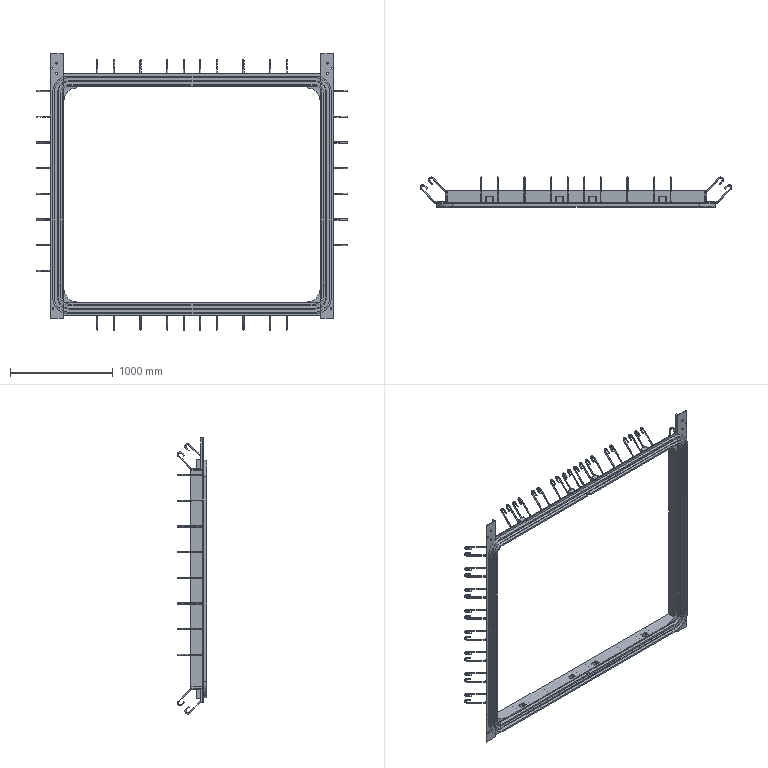Part | SolidWorks | features ReferencePattern 81, MirrorCompFeat 5, LocalLPattern 4, CompositeCurve 1 | 113 solids | 1210 faces | box 3027 x 288.723 x 2684 mm | volume 36409651 mm3 | cylinder 468 | plane 458 | torus 280 | spline 4 | commonest cylinder face diameters 12 x420 17.5 x28 130 x4 160 x4 240 x4 288 x4